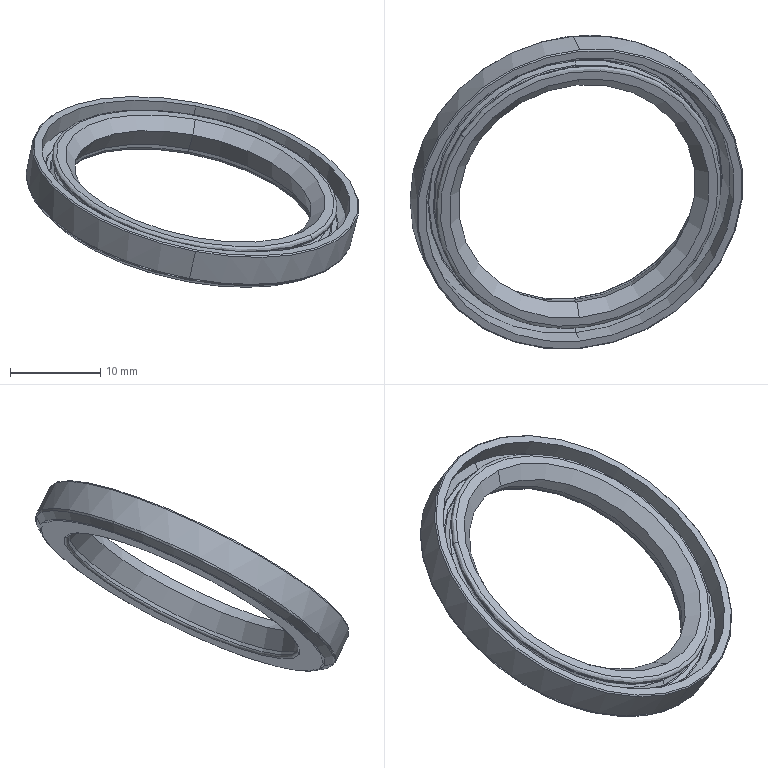Part | SolidWorks | features BaseBody 1 | 1 solid | 44 faces | box 36.935 x 34.817 x 21.16 mm | volume 1456 mm3 | spline 18 | cone 12 | cylinder 6 | torus 4 | plane 4 | commonest cylinder face diameters 28.6 x2 35 x2 37 x2